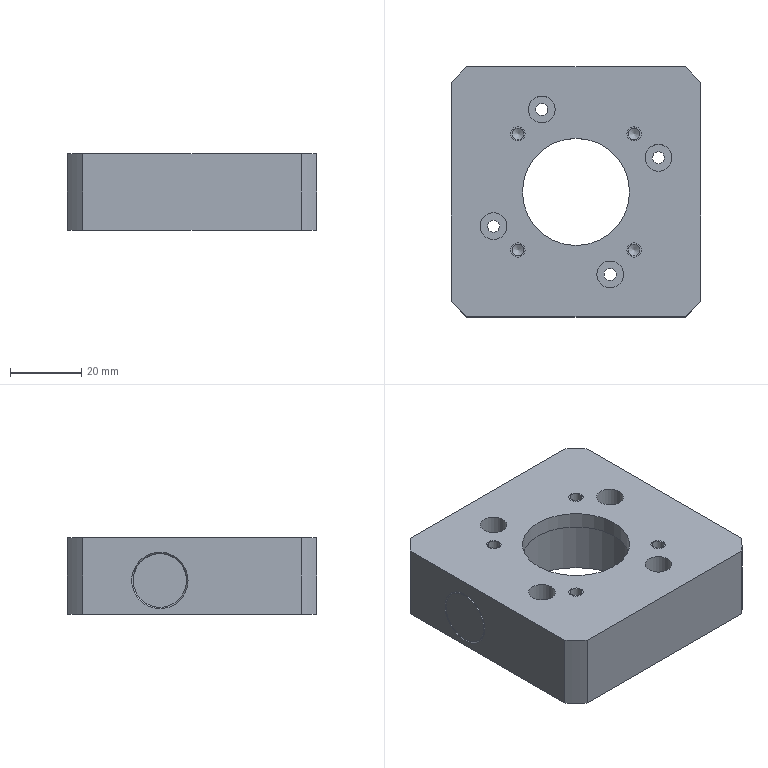Part | STEP file | P0409101803-0002 | 1 solid | 48 faces | box 70 x 70 x 21.5 mm | volume 78366 mm3 | cylinder 25 | plane 18 | cone 5 | commonest cylinder face diameters 3.3 x4 3.4 x4 4 x4 7.5 x4 93 x4 9 x1